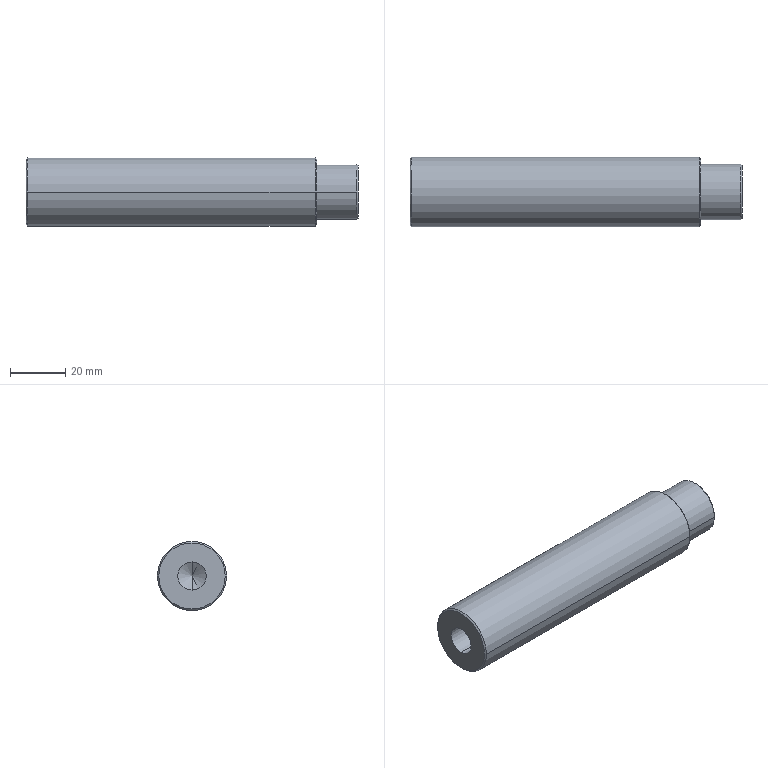Part | SolidWorks | features BaseBody 1 | 1 solid | 17 faces | box 120 x 25 x 25 mm | volume 53692 mm3 | cone 8 | cylinder 6 | plane 3 | commonest cylinder face diameters 10.2 x2 20 x2 25 x2
STEP:
#1=CARTESIAN_POINT('',(-30.,0.,-5.1));
#2=VERTEX_POINT('',#1);
#3=CARTESIAN_POINT('',(-30.,0.,5.1));
#4=VERTEX_POINT('',#3);
#5=CARTESIAN_POINT('',(-30.,0.,0.));
#6=DIRECTION('',(-1.,0.,0.));
#7=DIRECTION('',(0.,0.,1.));
#8=AXIS2_PLACEMENT_3D('',#5,#6,#7);
#9=CIRCLE('',#8,5.1);
#10=EDGE_CURVE('',#2,#4,#9,.T.);
#11=ORIENTED_EDGE('',*,*,#10,.F.);
#12=CARTESIAN_POINT('',(-60.,0.,-5.1));
#13=VERTEX_POINT('',#12);
#14=CARTESIAN_POINT('',(-60.,0.,-5.1));
#15=DIRECTION('',(-1.,0.,0.));
#16=VECTOR('',#15,1000.);
#17=LINE('',#14,#16);
#18=EDGE_CURVE('',#2,#13,#17,.T.);
#19=ORIENTED_EDGE('',*,*,#18,.T.);
#20=CARTESIAN_POINT('',(-60.,0.,5.1));
#21=VERTEX_POINT('',#20);
#22=CARTESIAN_POINT('',(-60.,0.,0.));
#23=DIRECTION('',(-1.,0.,0.));
#24=DIRECTION('',(0.,0.,1.));
#25=AXIS2_PLACEMENT_3D('',#22,#23,#24);
#26=CIRCLE('',#25,5.1);
#27=EDGE_CURVE('',#13,#21,#26,.T.);
#28=ORIENTED_EDGE('',*,*,#27,.T.);
#29=CARTESIAN_POINT('',(-60.,0.,5.1));
#30=DIRECTION('',(-1.,0.,0.));
#31=VECTOR('',#30,1000.);
#32=LINE('',#29,#31);
#33=EDGE_CURVE('',#4,#21,#32,.T.);
#34=ORIENTED_EDGE('',*,*,#33,.F.);
#35=EDGE_LOOP('',(#11,#19,#28,#34));
#36=FACE_OUTER_BOUND('',#35,.T.);
#37=CARTESIAN_POINT('',(-60.,0.,0.));
#38=DIRECTION('',(-1.,0.,0.));
#39=DIRECTION('',(0.,0.,1.));
#40=AXIS2_PLACEMENT_3D('',#37,#38,#39);
#41=CYLINDRICAL_SURFACE('',#40,5.1);
#42=ADVANCED_FACE('',(#36),#41,.F.);
#43=CARTESIAN_POINT('',(-26.936,0.,0.));
#44=VERTEX_POINT('',#43);
#45=CARTESIAN_POINT('',(-30.,0.,5.1));
#46=DIRECTION('',(-0.515,0.,0.8572));
#47=VECTOR('',#46,1000.);
#48=LINE('',#45,#47);
#49=EDGE_CURVE('',#44,#4,#48,.T.);
#50=ORIENTED_EDGE('',*,*,#49,.F.);
#51=CARTESIAN_POINT('',(-30.,0.,-5.1));
#52=DIRECTION('',(-0.515,0.,-0.8572));
#53=VECTOR('',#52,1000.);
#54=LINE('',#51,#53);
#55=EDGE_CURVE('',#44,#2,#54,.T.);
#56=ORIENTED_EDGE('',*,*,#55,.T.);
#57=ORIENTED_EDGE('',*,*,#10,.T.);
#58=EDGE_LOOP('',(#50,#56,#57));
#59=FACE_OUTER_BOUND('',#58,.T.);
#60=CARTESIAN_POINT('',(-30.,0.,0.));
#61=DIRECTION('',(-1.,0.,0.));
#62=DIRECTION('',(0.,0.,1.));
#63=AXIS2_PLACEMENT_3D('',#60,#61,#62);
#64=CONICAL_SURFACE('',#63,5.1,1.03);
#65=ADVANCED_FACE('',(#59),#64,.F.);
#66=CARTESIAN_POINT('',(60.,9.5,0.));
#67=VERTEX_POINT('',#66);
#68=CARTESIAN_POINT('',(60.,-9.5,0.));
#69=VERTEX_POINT('',#68);
#70=CARTESIAN_POINT('',(60.,0.,0.));
#71=DIRECTION('',(1.,0.,0.));
#72=DIRECTION('',(0.,-1.,0.));
#73=AXIS2_PLACEMENT_3D('',#70,#71,#72);
#74=CIRCLE('',#73,9.5);
#75=EDGE_CURVE('',#67,#69,#74,.T.);
#76=ORIENTED_EDGE('',*,*,#75,.F.);
#77=CARTESIAN_POINT('',(59.5,10.,0.));
#78=VERTEX_POINT('',#77);
#79=CARTESIAN_POINT('',(59.5,10.,0.));
#80=DIRECTION('',(-0.7071,0.7071,0.));
#81=VECTOR('',#80,1000.);
#82=LINE('',#79,#81);
#83=EDGE_CURVE('',#67,#78,#82,.T.);
#84=ORIENTED_EDGE('',*,*,#83,.T.);
#85=CARTESIAN_POINT('',(59.5,-10.,0.));
#86=VERTEX_POINT('',#85);
#87=CARTESIAN_POINT('',(59.5,0.,0.));
#88=DIRECTION('',(-1.,0.,0.));
#89=DIRECTION('',(0.,-1.,0.));
#90=AXIS2_PLACEMENT_3D('',#87,#88,#89);
#91=CIRCLE('',#90,10.);
#92=EDGE_CURVE('',#86,#78,#91,.T.);
#93=ORIENTED_EDGE('',*,*,#92,.F.);
#94=CARTESIAN_POINT('',(59.5,-10.,0.));
#95=DIRECTION('',(-0.7071,-0.7071,0.));
#96=VECTOR('',#95,1000.);
#97=LINE('',#94,#96);
#98=EDGE_CURVE('',#69,#86,#97,.T.);
#99=ORIENTED_EDGE('',*,*,#98,.F.);
#100=EDGE_LOOP('',(#76,#84,#93,#99));
#101=FACE_OUTER_BOUND('',#100,.T.);
#102=CARTESIAN_POINT('',(59.5,0.,0.));
#103=DIRECTION('',(-1.,0.,0.));
#104=DIRECTION('',(0.,-1.,0.));
#105=AXIS2_PLACEMENT_3D('',#102,#103,#104);
#106=CONICAL_SURFACE('',#105,10.,0.7854);
#107=ADVANCED_FACE('',(#101),#106,.T.);
#108=CARTESIAN_POINT('',(45.,12.,0.));
#109=VERTEX_POINT('',#108);
#110=CARTESIAN_POINT('',(45.,-12.,0.));
#111=VERTEX_POINT('',#110);
#112=CARTESIAN_POINT('',(45.,0.,0.));
#113=DIRECTION('',(1.,0.,0.));
#114=DIRECTION('',(0.,-1.,0.));
#115=AXIS2_PLACEMENT_3D('',#112,#113,#114);
#116=CIRCLE('',#115,12.);
#117=EDGE_CURVE('',#109,#111,#116,.T.);
#118=ORIENTED_EDGE('',*,*,#117,.F.);
#119=CARTESIAN_POINT('',(44.5,12.5,0.));
#120=VERTEX_POINT('',#119);
#121=CARTESIAN_POINT('',(44.5,12.5,0.));
#122=DIRECTION('',(-0.7071,0.7071,0.));
#123=VECTOR('',#122,1000.);
#124=LINE('',#121,#123);
#125=EDGE_CURVE('',#109,#120,#124,.T.);
#126=ORIENTED_EDGE('',*,*,#125,.T.);
#127=CARTESIAN_POINT('',(44.5,-12.5,0.));
#128=VERTEX_POINT('',#127);
#129=CARTESIAN_POINT('',(44.5,0.,0.));
#130=DIRECTION('',(-1.,0.,0.));
#131=DIRECTION('',(0.,-1.,0.));
#132=AXIS2_PLACEMENT_3D('',#129,#130,#131);
#133=CIRCLE('',#132,12.5);
#134=EDGE_CURVE('',#128,#120,#133,.T.);
#135=ORIENTED_EDGE('',*,*,#134,.F.);
#136=CARTESIAN_POINT('',(44.5,-12.5,0.));
#137=DIRECTION('',(-0.7071,-0.7071,0.));
#138=VECTOR('',#137,1000.);
#139=LINE('',#136,#138);
#140=EDGE_CURVE('',#111,#128,#139,.T.);
#141=ORIENTED_EDGE('',*,*,#140,.F.);
#142=EDGE_LOOP('',(#118,#126,#135,#141));
#143=FACE_OUTER_BOUND('',#142,.T.);
#144=CARTESIAN_POINT('',(44.5,0.,0.));
#145=DIRECTION('',(-1.,0.,0.));
#146=DIRECTION('',(0.,-1.,0.));
#147=AXIS2_PLACEMENT_3D('',#144,#145,#146);
#148=CONICAL_SURFACE('',#147,12.5,0.7854);
#149=ADVANCED_FACE('',(#143),#148,.T.);
#150=CARTESIAN_POINT('',(-60.,-12.,0.));
#151=VERTEX_POINT('',#150);
#152=CARTESIAN_POINT('',(-60.,12.,0.));
#153=VERTEX_POINT('',#152);
#154=CARTESIAN_POINT('',(-60.,0.,0.));
#155=DIRECTION('',(-1.,0.,0.));
#156=DIRECTION('',(0.,1.,0.));
#157=AXIS2_PLACEMENT_3D('',#154,#155,#156);
#158=CIRCLE('',#157,12.);
#159=EDGE_CURVE('',#151,#153,#158,.T.);
#160=ORIENTED_EDGE('',*,*,#159,.F.);
#161=CARTESIAN_POINT('',(-59.5,-12.5,0.));
#162=VERTEX_POINT('',#161);
#163=CARTESIAN_POINT('',(-60.,-12.,0.));
#164=DIRECTION('',(0.7071,-0.7071,0.));
#165=VECTOR('',#164,1000.);
#166=LINE('',#163,#165);
#167=EDGE_CURVE('',#151,#162,#166,.T.);
#168=ORIENTED_EDGE('',*,*,#167,.T.);
#169=CARTESIAN_POINT('',(-59.5,12.5,0.));
#170=VERTEX_POINT('',#169);
#171=CARTESIAN_POINT('',(-59.5,0.,0.));
#172=DIRECTION('',(1.,0.,0.));
#173=DIRECTION('',(0.,1.,0.));
#174=AXIS2_PLACEMENT_3D('',#171,#172,#173);
#175=CIRCLE('',#174,12.5);
#176=EDGE_CURVE('',#170,#162,#175,.T.);
#177=ORIENTED_EDGE('',*,*,#176,.F.);
#178=CARTESIAN_POINT('',(-60.,12.,0.));
#179=DIRECTION('',(0.7071,0.7071,0.));
#180=VECTOR('',#179,1000.);
#181=LINE('',#178,#180);
#182=EDGE_CURVE('',#153,#170,#181,.T.);
#183=ORIENTED_EDGE('',*,*,#182,.F.);
#184=EDGE_LOOP('',(#160,#168,#177,#183));
#185=FACE_OUTER_BOUND('',#184,.T.);
#186=CARTESIAN_POINT('',(-60.,0.,0.));
#187=DIRECTION('',(1.,0.,0.));
#188=DIRECTION('',(0.,1.,0.));
#189=AXIS2_PLACEMENT_3D('',#186,#187,#188);
#190=CONICAL_SURFACE('',#189,12.,0.7854);
#191=ADVANCED_FACE('',(#185),#190,.T.);
#192=ORIENTED_EDGE('',*,*,#134,.T.);
#193=CARTESIAN_POINT('',(-60.,12.5,0.));
#194=DIRECTION('',(-1.,0.,0.));
#195=VECTOR('',#194,1000.);
#196=LINE('',#193,#195);
#197=EDGE_CURVE('',#120,#170,#196,.T.);
#198=ORIENTED_EDGE('',*,*,#197,.T.);
#199=ORIENTED_EDGE('',*,*,#176,.T.);
#200=CARTESIAN_POINT('',(-60.,-12.5,0.));
#201=DIRECTION('',(-1.,0.,0.));
#202=VECTOR('',#201,1000.);
#203=LINE('',#200,#202);
#204=EDGE_CURVE('',#128,#162,#203,.T.);
#205=ORIENTED_EDGE('',*,*,#204,.F.);
#206=EDGE_LOOP('',(#192,#198,#199,#205));
#207=FACE_OUTER_BOUND('',#206,.T.);
#208=CARTESIAN_POINT('',(-60.,0.,0.));
#209=DIRECTION('',(-1.,0.,0.));
#210=DIRECTION('',(0.,-1.,0.));
#211=AXIS2_PLACEMENT_3D('',#208,#209,#210);
#212=CYLINDRICAL_SURFACE('',#211,12.5);
#213=ADVANCED_FACE('',(#207),#212,.T.);
#214=ORIENTED_EDGE('',*,*,#92,.T.);
#215=CARTESIAN_POINT('',(45.,10.,0.));
#216=VERTEX_POINT('',#215);
#217=CARTESIAN_POINT('',(-60.,10.,0.));
#218=DIRECTION('',(-1.,0.,0.));
#219=VECTOR('',#218,1000.);
#220=LINE('',#217,#219);
#221=EDGE_CURVE('',#78,#216,#220,.T.);
#222=ORIENTED_EDGE('',*,*,#221,.T.);
#223=CARTESIAN_POINT('',(45.,-10.,0.));
#224=VERTEX_POINT('',#223);
#225=CARTESIAN_POINT('',(45.,0.,0.));
#226=DIRECTION('',(-1.,0.,0.));
#227=DIRECTION('',(0.,-1.,0.));
#228=AXIS2_PLACEMENT_3D('',#225,#226,#227);
#229=CIRCLE('',#228,10.);
#230=EDGE_CURVE('',#224,#216,#229,.T.);
#231=ORIENTED_EDGE('',*,*,#230,.F.);
#232=CARTESIAN_POINT('',(-60.,-10.,0.));
#233=DIRECTION('',(-1.,0.,0.));
#234=VECTOR('',#233,1000.);
#235=LINE('',#232,#234);
#236=EDGE_CURVE('',#86,#224,#235,.T.);
#237=ORIENTED_EDGE('',*,*,#236,.F.);
#238=EDGE_LOOP('',(#214,#222,#231,#237));
#239=FACE_OUTER_BOUND('',#238,.T.);
#240=CARTESIAN_POINT('',(-60.,0.,0.));
#241=DIRECTION('',(-1.,0.,0.));
#242=DIRECTION('',(0.,-1.,0.));
#243=AXIS2_PLACEMENT_3D('',#240,#241,#242);
#244=CYLINDRICAL_SURFACE('',#243,10.);
#245=ADVANCED_FACE('',(#239),#244,.T.);
#246=CARTESIAN_POINT('',(60.,0.,0.));
#247=DIRECTION('',(1.,0.,0.));
#248=DIRECTION('',(0.,-1.,0.));
#249=AXIS2_PLACEMENT_3D('',#246,#247,#248);
#250=CIRCLE('',#249,9.5);
#251=EDGE_CURVE('',#69,#67,#250,.T.);
#252=ORIENTED_EDGE('',*,*,#251,.T.);
#253=ORIENTED_EDGE('',*,*,#75,.T.);
#254=EDGE_LOOP('',(#252,#253));
#255=FACE_OUTER_BOUND('',#254,.T.);
#256=CARTESIAN_POINT('',(60.,10.,0.));
#257=DIRECTION('',(-1.,0.,0.));
#258=DIRECTION('',(0.,-1.,0.));
#259=AXIS2_PLACEMENT_3D('',#256,#257,#258);
#260=PLANE('',#259);
#261=ADVANCED_FACE('',(#255),#260,.F.);
#262=ORIENTED_EDGE('',*,*,#221,.F.);
#263=CARTESIAN_POINT('',(59.5,0.,0.));
#264=DIRECTION('',(-1.,0.,0.));
#265=DIRECTION('',(0.,-1.,0.));
#266=AXIS2_PLACEMENT_3D('',#263,#264,#265);
#267=CIRCLE('',#266,10.);
#268=EDGE_CURVE('',#78,#86,#267,.T.);
#269=ORIENTED_EDGE('',*,*,#268,.T.);
#270=ORIENTED_EDGE('',*,*,#236,.T.);
#271=CARTESIAN_POINT('',(45.,0.,0.));
#272=DIRECTION('',(-1.,0.,0.));
#273=DIRECTION('',(0.,-1.,0.));
#274=AXIS2_PLACEMENT_3D('',#271,#272,#273);
#275=CIRCLE('',#274,10.);
#276=EDGE_CURVE('',#216,#224,#275,.T.);
#277=ORIENTED_EDGE('',*,*,#276,.F.);
#278=EDGE_LOOP('',(#262,#269,#270,#277));
#279=FACE_OUTER_BOUND('',#278,.T.);
#280=CARTESIAN_POINT('',(-60.,0.,0.));
#281=DIRECTION('',(-1.,0.,0.));
#282=DIRECTION('',(0.,-1.,0.));
#283=AXIS2_PLACEMENT_3D('',#280,#281,#282);
#284=CYLINDRICAL_SURFACE('',#283,10.);
#285=ADVANCED_FACE('',(#279),#284,.T.);
#286=CARTESIAN_POINT('',(45.,0.,0.));
#287=DIRECTION('',(1.,0.,0.));
#288=DIRECTION('',(0.,-1.,0.));
#289=AXIS2_PLACEMENT_3D('',#286,#287,#288);
#290=CIRCLE('',#289,12.);
#291=EDGE_CURVE('',#111,#109,#290,.T.);
#292=ORIENTED_EDGE('',*,*,#291,.T.);
#293=ORIENTED_EDGE('',*,*,#117,.T.);
#294=EDGE_LOOP('',(#292,#293));
#295=FACE_OUTER_BOUND('',#294,.T.);
#296=ORIENTED_EDGE('',*,*,#230,.T.);
#297=ORIENTED_EDGE('',*,*,#276,.T.);
#298=EDGE_LOOP('',(#296,#297));
#299=FACE_BOUND('',#298,.T.);
#300=CARTESIAN_POINT('',(45.,12.5,0.));
#301=DIRECTION('',(-1.,0.,0.));
#302=DIRECTION('',(0.,-1.,0.));
#303=AXIS2_PLACEMENT_3D('',#300,#301,#302);
#304=PLANE('',#303);
#305=ADVANCED_FACE('',(#295,#299),#304,.F.);
#306=ORIENTED_EDGE('',*,*,#197,.F.);
#307=CARTESIAN_POINT('',(44.5,0.,0.));
#308=DIRECTION('',(-1.,0.,0.));
#309=DIRECTION('',(0.,-1.,0.));
#310=AXIS2_PLACEMENT_3D('',#307,#308,#309);
#311=CIRCLE('',#310,12.5);
#312=EDGE_CURVE('',#120,#128,#311,.T.);
#313=ORIENTED_EDGE('',*,*,#312,.T.);
#314=ORIENTED_EDGE('',*,*,#204,.T.);
#315=CARTESIAN_POINT('',(-59.5,0.,0.));
#316=DIRECTION('',(1.,0.,0.));
#317=DIRECTION('',(0.,1.,0.));
#318=AXIS2_PLACEMENT_3D('',#315,#316,#317);
#319=CIRCLE('',#318,12.5);
#320=EDGE_CURVE('',#162,#170,#319,.T.);
#321=ORIENTED_EDGE('',*,*,#320,.T.);
#322=EDGE_LOOP('',(#306,#313,#314,#321));
#323=FACE_OUTER_BOUND('',#322,.T.);
#324=CARTESIAN_POINT('',(-60.,0.,0.));
#325=DIRECTION('',(-1.,0.,0.));
#326=DIRECTION('',(0.,-1.,0.));
#327=AXIS2_PLACEMENT_3D('',#324,#325,#326);
#328=CYLINDRICAL_SURFACE('',#327,12.5);
#329=ADVANCED_FACE('',(#323),#328,.T.);
#330=CARTESIAN_POINT('',(-60.,0.,0.));
#331=DIRECTION('',(-1.,0.,0.));
#332=DIRECTION('',(0.,0.,1.));
#333=AXIS2_PLACEMENT_3D('',#330,#331,#332);
#334=CIRCLE('',#333,5.1);
#335=EDGE_CURVE('',#21,#13,#334,.T.);
#336=ORIENTED_EDGE('',*,*,#335,.F.);
#337=ORIENTED_EDGE('',*,*,#27,.F.);
#338=EDGE_LOOP('',(#336,#337));
#339=FACE_BOUND('',#338,.T.);
#340=CARTESIAN_POINT('',(-60.,0.,0.));
#341=DIRECTION('',(-1.,0.,0.));
#342=DIRECTION('',(0.,1.,0.));
#343=AXIS2_PLACEMENT_3D('',#340,#341,#342);
#344=CIRCLE('',#343,12.);
#345=EDGE_CURVE('',#153,#151,#344,.T.);
#346=ORIENTED_EDGE('',*,*,#345,.T.);
#347=ORIENTED_EDGE('',*,*,#159,.T.);
#348=EDGE_LOOP('',(#346,#347));
#349=FACE_OUTER_BOUND('',#348,.T.);
#350=CARTESIAN_POINT('',(-60.,0.,0.));
#351=DIRECTION('',(1.,0.,0.));
#352=DIRECTION('',(0.,1.,0.));
#353=AXIS2_PLACEMENT_3D('',#350,#351,#352);
#354=PLANE('',#353);
#355=ADVANCED_FACE('',(#339,#349),#354,.F.);
#356=ORIENTED_EDGE('',*,*,#167,.F.);
#357=ORIENTED_EDGE('',*,*,#345,.F.);
#358=ORIENTED_EDGE('',*,*,#182,.T.);
#359=ORIENTED_EDGE('',*,*,#320,.F.);
#360=EDGE_LOOP('',(#356,#357,#358,#359));
#361=FACE_OUTER_BOUND('',#360,.T.);
#362=CARTESIAN_POINT('',(-60.,0.,0.));
#363=DIRECTION('',(1.,0.,0.));
#364=DIRECTION('',(0.,1.,0.));
#365=AXIS2_PLACEMENT_3D('',#362,#363,#364);
#366=CONICAL_SURFACE('',#365,12.,0.7854);
#367=ADVANCED_FACE('',(#361),#366,.T.);
#368=ORIENTED_EDGE('',*,*,#125,.F.);
#369=ORIENTED_EDGE('',*,*,#291,.F.);
#370=ORIENTED_EDGE('',*,*,#140,.T.);
#371=ORIENTED_EDGE('',*,*,#312,.F.);
#372=EDGE_LOOP('',(#368,#369,#370,#371));
#373=FACE_OUTER_BOUND('',#372,.T.);
#374=CARTESIAN_POINT('',(44.5,0.,0.));
#375=DIRECTION('',(-1.,0.,0.));
#376=DIRECTION('',(0.,-1.,0.));
#377=AXIS2_PLACEMENT_3D('',#374,#375,#376);
#378=CONICAL_SURFACE('',#377,12.5,0.7854);
#379=ADVANCED_FACE('',(#373),#378,.T.);
#380=ORIENTED_EDGE('',*,*,#83,.F.);
#381=ORIENTED_EDGE('',*,*,#251,.F.);
#382=ORIENTED_EDGE('',*,*,#98,.T.);
#383=ORIENTED_EDGE('',*,*,#268,.F.);
#384=EDGE_LOOP('',(#380,#381,#382,#383));
#385=FACE_OUTER_BOUND('',#384,.T.);
#386=CARTESIAN_POINT('',(59.5,0.,0.));
#387=DIRECTION('',(-1.,0.,0.));
#388=DIRECTION('',(0.,-1.,0.));
#389=AXIS2_PLACEMENT_3D('',#386,#387,#388);
#390=CONICAL_SURFACE('',#389,10.,0.7854);
#391=ADVANCED_FACE('',(#385),#390,.T.);
#392=ORIENTED_EDGE('',*,*,#55,.F.);
#393=ORIENTED_EDGE('',*,*,#49,.T.);
#394=CARTESIAN_POINT('',(-30.,0.,0.));
#395=DIRECTION('',(-1.,0.,0.));
#396=DIRECTION('',(0.,0.,1.));
#397=AXIS2_PLACEMENT_3D('',#394,#395,#396);
#398=CIRCLE('',#397,5.1);
#399=EDGE_CURVE('',#4,#2,#398,.T.);
#400=ORIENTED_EDGE('',*,*,#399,.T.);
#401=EDGE_LOOP('',(#392,#393,#400));
#402=FACE_OUTER_BOUND('',#401,.T.);
#403=CARTESIAN_POINT('',(-30.,0.,0.));
#404=DIRECTION('',(-1.,0.,0.));
#405=DIRECTION('',(0.,0.,1.));
#406=AXIS2_PLACEMENT_3D('',#403,#404,#405);
#407=CONICAL_SURFACE('',#406,5.1,1.03);
#408=ADVANCED_FACE('',(#402),#407,.F.);
#409=ORIENTED_EDGE('',*,*,#18,.F.);
#410=ORIENTED_EDGE('',*,*,#399,.F.);
#411=ORIENTED_EDGE('',*,*,#33,.T.);
#412=ORIENTED_EDGE('',*,*,#335,.T.);
#413=EDGE_LOOP('',(#409,#410,#411,#412));
#414=FACE_OUTER_BOUND('',#413,.T.);
#415=CARTESIAN_POINT('',(-60.,0.,0.));
#416=DIRECTION('',(-1.,0.,0.));
#417=DIRECTION('',(0.,0.,1.));
#418=AXIS2_PLACEMENT_3D('',#415,#416,#417);
#419=CYLINDRICAL_SURFACE('',#418,5.1);
#420=ADVANCED_FACE('',(#414),#419,.F.);
#421=CLOSED_SHELL('',(#42,#65,#107,#149,#191,#213,#245,#261,#285,#305,#329,#355,#367,#379,#391,#408,#420));
#422=MANIFOLD_SOLID_BREP('',#421);
#423=CARTESIAN_POINT('',(0.,0.,0.));
#424=DIRECTION('',(0.,0.,1.));
#425=DIRECTION('',(1.,0.,0.));
#426=AXIS2_PLACEMENT_3D('',#423,#424,#425);
#427=(LENGTH_UNIT()NAMED_UNIT(*)SI_UNIT(.MILLI.,.METRE.));
#428=UNCERTAINTY_MEASURE_WITH_UNIT(LENGTH_MEASURE(0.00001),#427,'','');
#429=(NAMED_UNIT(*)PLANE_ANGLE_UNIT()SI_UNIT($,.RADIAN.));
#430=(NAMED_UNIT(*)SI_UNIT($,.STERADIAN.)SOLID_ANGLE_UNIT());
#431=(GEOMETRIC_REPRESENTATION_CONTEXT(3)GLOBAL_UNCERTAINTY_ASSIGNED_CONTEXT((#428))GLOBAL_UNIT_ASSIGNED_CONTEXT((#427,#429,#430))REPRESENTATION_CONTEXT('',''));
#432=ADVANCED_BREP_SHAPE_REPRESENTATION('',(#422,#426),#431);